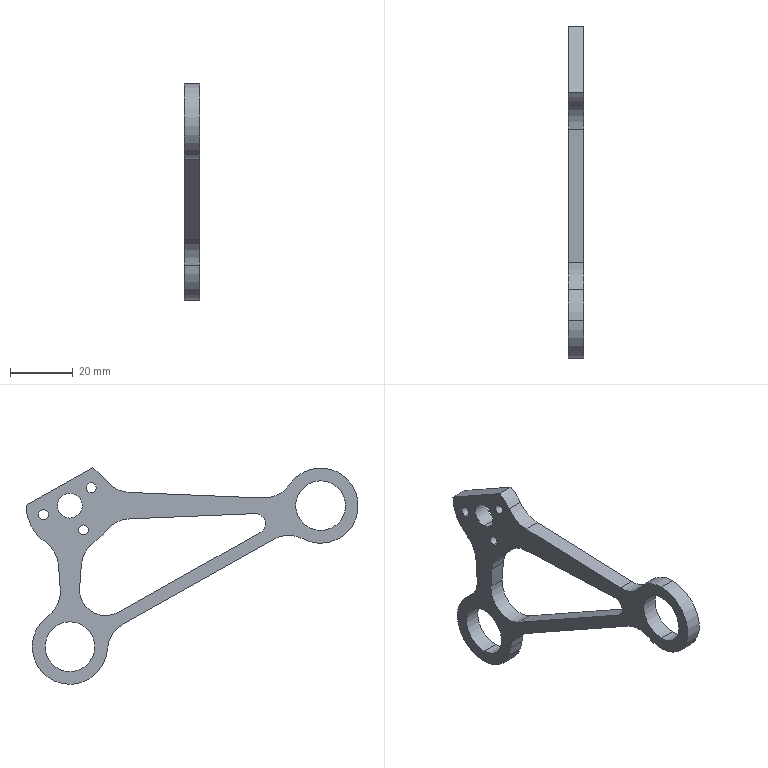Part | SolidWorks | features BaseBody 1 | 1 solid | 40 faces | box 5.08 x 106 x 69.07 mm | volume 9043 mm3 | cylinder 31 | plane 9 | commonest cylinder face diameters 20 x9 3.175 x6 15.875 x4 24 x4 28 x3 6.399 x2
STEP:
#1=CARTESIAN_POINT('',(-2.54,-4.358,-9.336));
#2=VERTEX_POINT('',#1);
#3=CARTESIAN_POINT('',(-2.54,-4.358,-6.161));
#4=VERTEX_POINT('',#3);
#5=CARTESIAN_POINT('',(-2.54,-4.358,-7.748));
#6=DIRECTION('',(-1.,0.,0.));
#7=DIRECTION('',(0.,0.,-1.));
#8=AXIS2_PLACEMENT_3D('',#5,#6,#7);
#9=CIRCLE('',#8,1.588);
#10=EDGE_CURVE('',#2,#4,#9,.T.);
#11=ORIENTED_EDGE('',*,*,#10,.T.);
#12=CARTESIAN_POINT('',(2.54,-4.358,-6.161));
#13=VERTEX_POINT('',#12);
#14=CARTESIAN_POINT('',(-2.54,-4.358,-6.161));
#15=DIRECTION('',(1.,0.,0.));
#16=VECTOR('',#15,1000.);
#17=LINE('',#14,#16);
#18=EDGE_CURVE('',#4,#13,#17,.T.);
#19=ORIENTED_EDGE('',*,*,#18,.T.);
#20=CARTESIAN_POINT('',(2.54,-4.358,-9.336));
#21=VERTEX_POINT('',#20);
#22=CARTESIAN_POINT('',(2.54,-4.358,-7.748));
#23=DIRECTION('',(1.,0.,0.));
#24=DIRECTION('',(0.,0.,-1.));
#25=AXIS2_PLACEMENT_3D('',#22,#23,#24);
#26=CIRCLE('',#25,1.588);
#27=EDGE_CURVE('',#13,#21,#26,.T.);
#28=ORIENTED_EDGE('',*,*,#27,.T.);
#29=CARTESIAN_POINT('',(-2.54,-4.358,-9.336));
#30=DIRECTION('',(1.,0.,0.));
#31=VECTOR('',#30,1000.);
#32=LINE('',#29,#31);
#33=EDGE_CURVE('',#2,#21,#32,.T.);
#34=ORIENTED_EDGE('',*,*,#33,.F.);
#35=EDGE_LOOP('',(#11,#19,#28,#34));
#36=FACE_OUTER_BOUND('',#35,.T.);
#37=CARTESIAN_POINT('',(-2.54,-4.358,-7.748));
#38=DIRECTION('',(1.,0.,0.));
#39=DIRECTION('',(0.,0.,-1.));
#40=AXIS2_PLACEMENT_3D('',#37,#38,#39);
#41=CYLINDRICAL_SURFACE('',#40,1.588);
#42=ADVANCED_FACE('',(#36),#41,.F.);
#43=CARTESIAN_POINT('',(2.54,0.,-52.937));
#44=VERTEX_POINT('',#43);
#45=CARTESIAN_POINT('',(2.54,0.,-37.063));
#46=VERTEX_POINT('',#45);
#47=CARTESIAN_POINT('',(2.54,0.,-45.));
#48=DIRECTION('',(-1.,0.,0.));
#49=DIRECTION('',(0.,0.,1.));
#50=AXIS2_PLACEMENT_3D('',#47,#48,#49);
#51=CIRCLE('',#50,7.937);
#52=EDGE_CURVE('',#44,#46,#51,.T.);
#53=ORIENTED_EDGE('',*,*,#52,.F.);
#54=CARTESIAN_POINT('',(-2.54,0.,-52.937));
#55=VERTEX_POINT('',#54);
#56=CARTESIAN_POINT('',(2.54,0.,-52.937));
#57=DIRECTION('',(-1.,0.,0.));
#58=VECTOR('',#57,1000.);
#59=LINE('',#56,#58);
#60=EDGE_CURVE('',#44,#55,#59,.T.);
#61=ORIENTED_EDGE('',*,*,#60,.T.);
#62=CARTESIAN_POINT('',(-2.54,0.,-37.063));
#63=VERTEX_POINT('',#62);
#64=CARTESIAN_POINT('',(-2.54,0.,-45.));
#65=DIRECTION('',(-1.,0.,0.));
#66=DIRECTION('',(0.,0.,1.));
#67=AXIS2_PLACEMENT_3D('',#64,#65,#66);
#68=CIRCLE('',#67,7.937);
#69=EDGE_CURVE('',#55,#63,#68,.T.);
#70=ORIENTED_EDGE('',*,*,#69,.T.);
#71=CARTESIAN_POINT('',(2.54,0.,-37.063));
#72=DIRECTION('',(-1.,0.,0.));
#73=VECTOR('',#72,1000.);
#74=LINE('',#71,#73);
#75=EDGE_CURVE('',#46,#63,#74,.T.);
#76=ORIENTED_EDGE('',*,*,#75,.F.);
#77=EDGE_LOOP('',(#53,#61,#70,#76));
#78=FACE_OUTER_BOUND('',#77,.T.);
#79=CARTESIAN_POINT('',(2.54,0.,-45.));
#80=DIRECTION('',(-1.,0.,0.));
#81=DIRECTION('',(0.,0.,1.));
#82=AXIS2_PLACEMENT_3D('',#79,#80,#81);
#83=CYLINDRICAL_SURFACE('',#82,7.937);
#84=ADVANCED_FACE('',(#78),#83,.F.);
#85=CARTESIAN_POINT('',(2.54,0.,-3.969));
#86=VERTEX_POINT('',#85);
#87=CARTESIAN_POINT('',(2.54,0.,3.969));
#88=VERTEX_POINT('',#87);
#89=CARTESIAN_POINT('',(2.54,0.,0.));
#90=DIRECTION('',(-1.,0.,0.));
#91=DIRECTION('',(0.,0.,1.));
#92=AXIS2_PLACEMENT_3D('',#89,#90,#91);
#93=CIRCLE('',#92,3.969);
#94=EDGE_CURVE('',#86,#88,#93,.T.);
#95=ORIENTED_EDGE('',*,*,#94,.F.);
#96=CARTESIAN_POINT('',(-2.54,0.,-3.969));
#97=VERTEX_POINT('',#96);
#98=CARTESIAN_POINT('',(2.54,0.,-3.969));
#99=DIRECTION('',(-1.,0.,0.));
#100=VECTOR('',#99,1000.);
#101=LINE('',#98,#100);
#102=EDGE_CURVE('',#86,#97,#101,.T.);
#103=ORIENTED_EDGE('',*,*,#102,.T.);
#104=CARTESIAN_POINT('',(-2.54,0.,3.969));
#105=VERTEX_POINT('',#104);
#106=CARTESIAN_POINT('',(-2.54,0.,0.));
#107=DIRECTION('',(-1.,0.,0.));
#108=DIRECTION('',(0.,0.,1.));
#109=AXIS2_PLACEMENT_3D('',#106,#107,#108);
#110=CIRCLE('',#109,3.969);
#111=EDGE_CURVE('',#97,#105,#110,.T.);
#112=ORIENTED_EDGE('',*,*,#111,.T.);
#113=CARTESIAN_POINT('',(2.54,0.,3.969));
#114=DIRECTION('',(-1.,0.,0.));
#115=VECTOR('',#114,1000.);
#116=LINE('',#113,#115);
#117=EDGE_CURVE('',#88,#105,#116,.T.);
#118=ORIENTED_EDGE('',*,*,#117,.F.);
#119=EDGE_LOOP('',(#95,#103,#112,#118));
#120=FACE_OUTER_BOUND('',#119,.T.);
#121=CARTESIAN_POINT('',(2.54,0.,0.));
#122=DIRECTION('',(-1.,0.,0.));
#123=DIRECTION('',(0.,0.,1.));
#124=AXIS2_PLACEMENT_3D('',#121,#122,#123);
#125=CYLINDRICAL_SURFACE('',#124,3.969);
#126=ADVANCED_FACE('',(#120),#125,.F.);
#127=CARTESIAN_POINT('',(2.54,-59.175,-2.55));
#128=VERTEX_POINT('',#127);
#129=CARTESIAN_POINT('',(2.54,-59.042,-2.552));
#130=VERTEX_POINT('',#129);
#131=CARTESIAN_POINT('',(2.54,-59.175,-5.749));
#132=DIRECTION('',(-1.,0.,0.));
#133=DIRECTION('',(0.,0.,1.));
#134=AXIS2_PLACEMENT_3D('',#131,#132,#133);
#135=CIRCLE('',#134,3.199);
#136=EDGE_CURVE('',#128,#130,#135,.T.);
#137=ORIENTED_EDGE('',*,*,#136,.F.);
#138=CARTESIAN_POINT('',(-2.54,-59.175,-2.55));
#139=VERTEX_POINT('',#138);
#140=CARTESIAN_POINT('',(2.54,-59.175,-2.55));
#141=DIRECTION('',(-1.,0.,0.));
#142=VECTOR('',#141,1000.);
#143=LINE('',#140,#142);
#144=EDGE_CURVE('',#128,#139,#143,.T.);
#145=ORIENTED_EDGE('',*,*,#144,.T.);
#146=CARTESIAN_POINT('',(-2.54,-59.042,-2.552));
#147=VERTEX_POINT('',#146);
#148=CARTESIAN_POINT('',(-2.54,-59.175,-5.749));
#149=DIRECTION('',(-1.,0.,0.));
#150=DIRECTION('',(0.,0.,1.));
#151=AXIS2_PLACEMENT_3D('',#148,#149,#150);
#152=CIRCLE('',#151,3.199);
#153=EDGE_CURVE('',#139,#147,#152,.T.);
#154=ORIENTED_EDGE('',*,*,#153,.T.);
#155=CARTESIAN_POINT('',(0.,-59.042,-2.552));
#156=DIRECTION('',(-1.,0.,0.));
#157=VECTOR('',#156,1000.);
#158=LINE('',#155,#157);
#159=EDGE_CURVE('',#130,#147,#158,.T.);
#160=ORIENTED_EDGE('',*,*,#159,.F.);
#161=EDGE_LOOP('',(#137,#145,#154,#160));
#162=FACE_OUTER_BOUND('',#161,.T.);
#163=CARTESIAN_POINT('',(2.54,-59.175,-5.749));
#164=DIRECTION('',(-1.,0.,0.));
#165=DIRECTION('',(0.,0.,1.));
#166=AXIS2_PLACEMENT_3D('',#163,#164,#165);
#167=CYLINDRICAL_SURFACE('',#166,3.199);
#168=ADVANCED_FACE('',(#162),#167,.F.);
#169=CARTESIAN_POINT('',(2.54,-80.,-7.938));
#170=VERTEX_POINT('',#169);
#171=CARTESIAN_POINT('',(2.54,-80.,7.938));
#172=VERTEX_POINT('',#171);
#173=CARTESIAN_POINT('',(2.54,-80.,0.));
#174=DIRECTION('',(-1.,0.,0.));
#175=DIRECTION('',(0.,0.,1.));
#176=AXIS2_PLACEMENT_3D('',#173,#174,#175);
#177=CIRCLE('',#176,7.938);
#178=EDGE_CURVE('',#170,#172,#177,.T.);
#179=ORIENTED_EDGE('',*,*,#178,.F.);
#180=CARTESIAN_POINT('',(-2.54,-80.,-7.938));
#181=VERTEX_POINT('',#180);
#182=CARTESIAN_POINT('',(2.54,-80.,-7.938));
#183=DIRECTION('',(-1.,0.,0.));
#184=VECTOR('',#183,1000.);
#185=LINE('',#182,#184);
#186=EDGE_CURVE('',#170,#181,#185,.T.);
#187=ORIENTED_EDGE('',*,*,#186,.T.);
#188=CARTESIAN_POINT('',(-2.54,-80.,7.938));
#189=VERTEX_POINT('',#188);
#190=CARTESIAN_POINT('',(-2.54,-80.,0.));
#191=DIRECTION('',(-1.,0.,0.));
#192=DIRECTION('',(0.,0.,1.));
#193=AXIS2_PLACEMENT_3D('',#190,#191,#192);
#194=CIRCLE('',#193,7.938);
#195=EDGE_CURVE('',#181,#189,#194,.T.);
#196=ORIENTED_EDGE('',*,*,#195,.T.);
#197=CARTESIAN_POINT('',(2.54,-80.,7.938));
#198=DIRECTION('',(-1.,0.,0.));
#199=VECTOR('',#198,1000.);
#200=LINE('',#197,#199);
#201=EDGE_CURVE('',#172,#189,#200,.T.);
#202=ORIENTED_EDGE('',*,*,#201,.F.);
#203=EDGE_LOOP('',(#179,#187,#196,#202));
#204=FACE_OUTER_BOUND('',#203,.T.);
#205=CARTESIAN_POINT('',(2.54,-80.,0.));
#206=DIRECTION('',(-1.,0.,0.));
#207=DIRECTION('',(0.,0.,1.));
#208=AXIS2_PLACEMENT_3D('',#205,#206,#207);
#209=CYLINDRICAL_SURFACE('',#208,7.938);
#210=ADVANCED_FACE('',(#204),#209,.F.);
#211=CARTESIAN_POINT('',(-2.54,-6.818,4.117));
#212=VERTEX_POINT('',#211);
#213=CARTESIAN_POINT('',(-2.54,-6.818,7.292));
#214=VERTEX_POINT('',#213);
#215=CARTESIAN_POINT('',(-2.54,-6.818,5.705));
#216=DIRECTION('',(-1.,0.,0.));
#217=DIRECTION('',(0.,0.,-1.));
#218=AXIS2_PLACEMENT_3D('',#215,#216,#217);
#219=CIRCLE('',#218,1.588);
#220=EDGE_CURVE('',#212,#214,#219,.T.);
#221=ORIENTED_EDGE('',*,*,#220,.T.);
#222=CARTESIAN_POINT('',(2.54,-6.818,7.292));
#223=VERTEX_POINT('',#222);
#224=CARTESIAN_POINT('',(-2.54,-6.818,7.292));
#225=DIRECTION('',(1.,0.,0.));
#226=VECTOR('',#225,1000.);
#227=LINE('',#224,#226);
#228=EDGE_CURVE('',#214,#223,#227,.T.);
#229=ORIENTED_EDGE('',*,*,#228,.T.);
#230=CARTESIAN_POINT('',(2.54,-6.818,4.117));
#231=VERTEX_POINT('',#230);
#232=CARTESIAN_POINT('',(2.54,-6.818,5.705));
#233=DIRECTION('',(-1.,0.,0.));
#234=DIRECTION('',(0.,0.,-1.));
#235=AXIS2_PLACEMENT_3D('',#232,#233,#234);
#236=CIRCLE('',#235,1.588);
#237=EDGE_CURVE('',#231,#223,#236,.T.);
#238=ORIENTED_EDGE('',*,*,#237,.F.);
#239=CARTESIAN_POINT('',(-2.54,-6.818,4.117));
#240=DIRECTION('',(1.,0.,0.));
#241=VECTOR('',#240,1000.);
#242=LINE('',#239,#241);
#243=EDGE_CURVE('',#212,#231,#242,.T.);
#244=ORIENTED_EDGE('',*,*,#243,.F.);
#245=EDGE_LOOP('',(#221,#229,#238,#244));
#246=FACE_OUTER_BOUND('',#245,.T.);
#247=CARTESIAN_POINT('',(-2.54,-6.818,5.705));
#248=DIRECTION('',(1.,0.,0.));
#249=DIRECTION('',(0.,0.,-1.));
#250=AXIS2_PLACEMENT_3D('',#247,#248,#249);
#251=CYLINDRICAL_SURFACE('',#250,1.588);
#252=ADVANCED_FACE('',(#246),#251,.F.);
#253=CARTESIAN_POINT('',(-2.54,8.416,-4.452));
#254=VERTEX_POINT('',#253);
#255=CARTESIAN_POINT('',(-2.54,8.416,-1.277));
#256=VERTEX_POINT('',#255);
#257=CARTESIAN_POINT('',(-2.54,8.416,-2.865));
#258=DIRECTION('',(-1.,0.,0.));
#259=DIRECTION('',(0.,0.,-1.));
#260=AXIS2_PLACEMENT_3D('',#257,#258,#259);
#261=CIRCLE('',#260,1.587);
#262=EDGE_CURVE('',#254,#256,#261,.T.);
#263=ORIENTED_EDGE('',*,*,#262,.T.);
#264=CARTESIAN_POINT('',(2.54,8.416,-1.277));
#265=VERTEX_POINT('',#264);
#266=CARTESIAN_POINT('',(-2.54,8.416,-1.277));
#267=DIRECTION('',(1.,0.,0.));
#268=VECTOR('',#267,1000.);
#269=LINE('',#266,#268);
#270=EDGE_CURVE('',#256,#265,#269,.T.);
#271=ORIENTED_EDGE('',*,*,#270,.T.);
#272=CARTESIAN_POINT('',(2.54,8.416,-4.452));
#273=VERTEX_POINT('',#272);
#274=CARTESIAN_POINT('',(2.54,8.416,-2.865));
#275=DIRECTION('',(-1.,0.,0.));
#276=DIRECTION('',(0.,0.,-1.));
#277=AXIS2_PLACEMENT_3D('',#274,#275,#276);
#278=CIRCLE('',#277,1.587);
#279=EDGE_CURVE('',#273,#265,#278,.T.);
#280=ORIENTED_EDGE('',*,*,#279,.F.);
#281=CARTESIAN_POINT('',(-2.54,8.416,-4.452));
#282=DIRECTION('',(1.,0.,0.));
#283=VECTOR('',#282,1000.);
#284=LINE('',#281,#283);
#285=EDGE_CURVE('',#254,#273,#284,.T.);
#286=ORIENTED_EDGE('',*,*,#285,.F.);
#287=EDGE_LOOP('',(#263,#271,#280,#286));
#288=FACE_OUTER_BOUND('',#287,.T.);
#289=CARTESIAN_POINT('',(-2.54,8.416,-2.865));
#290=DIRECTION('',(1.,0.,0.));
#291=DIRECTION('',(0.,0.,-1.));
#292=AXIS2_PLACEMENT_3D('',#289,#290,#291);
#293=CYLINDRICAL_SURFACE('',#292,1.587);
#294=ADVANCED_FACE('',(#288),#293,.F.);
#295=CARTESIAN_POINT('',(2.54,-69.812,-9.499));
#296=VERTEX_POINT('',#295);
#297=CARTESIAN_POINT('',(2.54,-64.909,-10.783));
#298=VERTEX_POINT('',#297);
#299=CARTESIAN_POINT('',(2.54,-69.812,-19.499));
#300=DIRECTION('',(-1.,0.,0.));
#301=DIRECTION('',(0.,0.,1.));
#302=AXIS2_PLACEMENT_3D('',#299,#300,#301);
#303=CIRCLE('',#302,10.);
#304=EDGE_CURVE('',#296,#298,#303,.T.);
#305=ORIENTED_EDGE('',*,*,#304,.F.);
#306=CARTESIAN_POINT('',(-2.54,-69.812,-9.499));
#307=VERTEX_POINT('',#306);
#308=CARTESIAN_POINT('',(2.54,-69.812,-9.499));
#309=DIRECTION('',(-1.,0.,0.));
#310=VECTOR('',#309,1000.);
#311=LINE('',#308,#310);
#312=EDGE_CURVE('',#296,#307,#311,.T.);
#313=ORIENTED_EDGE('',*,*,#312,.T.);
#314=CARTESIAN_POINT('',(-2.54,-64.909,-10.783));
#315=VERTEX_POINT('',#314);
#316=CARTESIAN_POINT('',(-2.54,-69.812,-19.499));
#317=DIRECTION('',(-1.,0.,0.));
#318=DIRECTION('',(0.,0.,1.));
#319=AXIS2_PLACEMENT_3D('',#316,#317,#318);
#320=CIRCLE('',#319,10.);
#321=EDGE_CURVE('',#307,#315,#320,.T.);
#322=ORIENTED_EDGE('',*,*,#321,.T.);
#323=CARTESIAN_POINT('',(0.,-64.909,-10.783));
#324=DIRECTION('',(1.,0.,0.));
#325=VECTOR('',#324,1000.);
#326=LINE('',#323,#325);
#327=EDGE_CURVE('',#315,#298,#326,.T.);
#328=ORIENTED_EDGE('',*,*,#327,.T.);
#329=EDGE_LOOP('',(#305,#313,#322,#328));
#330=FACE_OUTER_BOUND('',#329,.T.);
#331=CARTESIAN_POINT('',(2.54,-69.812,-19.499));
#332=DIRECTION('',(-1.,0.,0.));
#333=DIRECTION('',(0.,0.,1.));
#334=AXIS2_PLACEMENT_3D('',#331,#332,#333);
#335=CYLINDRICAL_SURFACE('',#334,10.);
#336=ADVANCED_FACE('',(#330),#335,.F.);
#337=CARTESIAN_POINT('',(2.54,-80.,-12.));
#338=VERTEX_POINT('',#337);
#339=CARTESIAN_POINT('',(2.54,-74.443,-10.636));
#340=VERTEX_POINT('',#339);
#341=CARTESIAN_POINT('',(2.54,-80.,0.));
#342=DIRECTION('',(1.,0.,0.));
#343=DIRECTION('',(0.,0.,1.));
#344=AXIS2_PLACEMENT_3D('',#341,#342,#343);
#345=CIRCLE('',#344,12.);
#346=EDGE_CURVE('',#338,#340,#345,.T.);
#347=ORIENTED_EDGE('',*,*,#346,.F.);
#348=CARTESIAN_POINT('',(-2.54,-80.,-12.));
#349=VERTEX_POINT('',#348);
#350=CARTESIAN_POINT('',(2.54,-80.,-12.));
#351=DIRECTION('',(-1.,0.,0.));
#352=VECTOR('',#351,1000.);
#353=LINE('',#350,#352);
#354=EDGE_CURVE('',#338,#349,#353,.T.);
#355=ORIENTED_EDGE('',*,*,#354,.T.);
#356=CARTESIAN_POINT('',(-2.54,-74.443,-10.636));
#357=VERTEX_POINT('',#356);
#358=CARTESIAN_POINT('',(-2.54,-80.,0.));
#359=DIRECTION('',(1.,0.,0.));
#360=DIRECTION('',(0.,0.,1.));
#361=AXIS2_PLACEMENT_3D('',#358,#359,#360);
#362=CIRCLE('',#361,12.);
#363=EDGE_CURVE('',#349,#357,#362,.T.);
#364=ORIENTED_EDGE('',*,*,#363,.T.);
#365=CARTESIAN_POINT('',(0.,-74.443,-10.636));
#366=DIRECTION('',(-1.,0.,0.));
#367=VECTOR('',#366,1000.);
#368=LINE('',#365,#367);
#369=EDGE_CURVE('',#340,#357,#368,.T.);
#370=ORIENTED_EDGE('',*,*,#369,.F.);
#371=EDGE_LOOP('',(#347,#355,#364,#370));
#372=FACE_OUTER_BOUND('',#371,.T.);
#373=CARTESIAN_POINT('',(2.54,-80.,0.));
#374=DIRECTION('',(-1.,0.,0.));
#375=DIRECTION('',(0.,0.,1.));
#376=AXIS2_PLACEMENT_3D('',#373,#374,#375);
#377=CYLINDRICAL_SURFACE('',#376,12.);
#378=ADVANCED_FACE('',(#372),#377,.T.);
#379=ORIENTED_EDGE('',*,*,#354,.F.);
#380=CARTESIAN_POINT('',(2.54,-80.,12.));
#381=VERTEX_POINT('',#380);
#382=CARTESIAN_POINT('',(2.54,-80.,0.));
#383=DIRECTION('',(1.,0.,0.));
#384=DIRECTION('',(0.,0.,1.));
#385=AXIS2_PLACEMENT_3D('',#382,#383,#384);
#386=CIRCLE('',#385,12.);
#387=EDGE_CURVE('',#381,#338,#386,.T.);
#388=ORIENTED_EDGE('',*,*,#387,.F.);
#389=CARTESIAN_POINT('',(-2.54,-80.,12.));
#390=VERTEX_POINT('',#389);
#391=CARTESIAN_POINT('',(2.54,-80.,12.));
#392=DIRECTION('',(-1.,0.,0.));
#393=VECTOR('',#392,1000.);
#394=LINE('',#391,#393);
#395=EDGE_CURVE('',#381,#390,#394,.T.);
#396=ORIENTED_EDGE('',*,*,#395,.T.);
#397=CARTESIAN_POINT('',(-2.54,-80.,0.));
#398=DIRECTION('',(1.,0.,0.));
#399=DIRECTION('',(0.,0.,1.));
#400=AXIS2_PLACEMENT_3D('',#397,#398,#399);
#401=CIRCLE('',#400,12.);
#402=EDGE_CURVE('',#390,#349,#401,.T.);
#403=ORIENTED_EDGE('',*,*,#402,.T.);
#404=EDGE_LOOP('',(#379,#388,#396,#403));
#405=FACE_OUTER_BOUND('',#404,.T.);
#406=CARTESIAN_POINT('',(2.54,-80.,0.));
#407=DIRECTION('',(-1.,0.,0.));
#408=DIRECTION('',(0.,0.,1.));
#409=AXIS2_PLACEMENT_3D('',#406,#407,#408);
#410=CYLINDRICAL_SURFACE('',#409,12.);
#411=ADVANCED_FACE('',(#405),#410,.T.);
#412=ORIENTED_EDGE('',*,*,#18,.F.);
#413=CARTESIAN_POINT('',(-2.54,-4.358,-7.748));
#414=DIRECTION('',(-1.,0.,0.));
#415=DIRECTION('',(0.,0.,-1.));
#416=AXIS2_PLACEMENT_3D('',#413,#414,#415);
#417=CIRCLE('',#416,1.588);
#418=EDGE_CURVE('',#4,#2,#417,.T.);
#419=ORIENTED_EDGE('',*,*,#418,.T.);
#420=ORIENTED_EDGE('',*,*,#33,.T.);
#421=CARTESIAN_POINT('',(2.54,-4.358,-7.748));
#422=DIRECTION('',(1.,0.,0.));
#423=DIRECTION('',(0.,0.,-1.));
#424=AXIS2_PLACEMENT_3D('',#421,#422,#423);
#425=CIRCLE('',#424,1.588);
#426=EDGE_CURVE('',#21,#13,#425,.T.);
#427=ORIENTED_EDGE('',*,*,#426,.T.);
#428=EDGE_LOOP('',(#412,#419,#420,#427));
#429=FACE_OUTER_BOUND('',#428,.T.);
#430=CARTESIAN_POINT('',(-2.54,-4.358,-7.748));
#431=DIRECTION('',(1.,0.,0.));
#432=DIRECTION('',(0.,0.,-1.));
#433=AXIS2_PLACEMENT_3D('',#430,#431,#432);
#434=CYLINDRICAL_SURFACE('',#433,1.588);
#435=ADVANCED_FACE('',(#429),#434,.F.);
#436=CARTESIAN_POINT('',(2.54,0.,-45.));
#437=DIRECTION('',(-1.,0.,0.));
#438=DIRECTION('',(0.,0.,1.));
#439=AXIS2_PLACEMENT_3D('',#436,#437,#438);
#440=CIRCLE('',#439,7.937);
#441=EDGE_CURVE('',#46,#44,#440,.T.);
#442=ORIENTED_EDGE('',*,*,#441,.T.);
#443=ORIENTED_EDGE('',*,*,#52,.T.);
#444=EDGE_LOOP('',(#442,#443));
#445=FACE_BOUND('',#444,.T.);
#446=CARTESIAN_POINT('',(2.54,0.,0.));
#447=DIRECTION('',(-1.,0.,0.));
#448=DIRECTION('',(0.,0.,1.));
#449=AXIS2_PLACEMENT_3D('',#446,#447,#448);
#450=CIRCLE('',#449,3.969);
#451=EDGE_CURVE('',#88,#86,#450,.T.);
#452=ORIENTED_EDGE('',*,*,#451,.T.);
#453=ORIENTED_EDGE('',*,*,#94,.T.);
#454=EDGE_LOOP('',(#452,#453));
#455=FACE_BOUND('',#454,.T.);
#456=CARTESIAN_POINT('',(2.54,-11.284,-8.287));
#457=VERTEX_POINT('',#456);
#458=CARTESIAN_POINT('',(2.54,-7.933,-11.536));
#459=VERTEX_POINT('',#458);
#460=CARTESIAN_POINT('',(2.54,0.,0.));
#461=DIRECTION('',(1.,0.,0.));
#462=DIRECTION('',(0.,0.,1.));
#463=AXIS2_PLACEMENT_3D('',#460,#461,#462);
#464=CIRCLE('',#463,14.);
#465=EDGE_CURVE('',#457,#459,#464,.T.);
#466=ORIENTED_EDGE('',*,*,#465,.T.);
#467=CARTESIAN_POINT('',(2.54,-3.625,-19.056));
#468=VERTEX_POINT('',#467);
#469=CARTESIAN_POINT('',(2.54,-13.599,-19.775));
#470=DIRECTION('',(-1.,0.,0.));
#471=DIRECTION('',(0.,0.,1.));
#472=AXIS2_PLACEMENT_3D('',#469,#470,#471);
#473=CIRCLE('',#472,10.);
#474=EDGE_CURVE('',#459,#468,#473,.T.);
#475=ORIENTED_EDGE('',*,*,#474,.T.);
#476=CARTESIAN_POINT('',(2.54,-3.11,-26.192));
#477=VERTEX_POINT('',#476);
#478=CARTESIAN_POINT('',(2.54,-3.625,-19.056));
#479=DIRECTION('',(0.,0.07196,-0.9974));
#480=VECTOR('',#479,1000.);
#481=LINE('',#478,#480);
#482=EDGE_CURVE('',#468,#477,#481,.T.);
#483=ORIENTED_EDGE('',*,*,#482,.T.);
#484=CARTESIAN_POINT('',(2.54,-15.447,-34.017));
#485=VERTEX_POINT('',#484);
#486=CARTESIAN_POINT('',(2.54,-11.381,-26.789));
#487=DIRECTION('',(-1.,0.,0.));
#488=DIRECTION('',(0.,0.,1.));
#489=AXIS2_PLACEMENT_3D('',#486,#487,#488);
#490=CIRCLE('',#489,8.292);
#491=EDGE_CURVE('',#477,#485,#490,.T.);
#492=ORIENTED_EDGE('',*,*,#491,.T.);
#493=CARTESIAN_POINT('',(2.54,-60.743,-8.537));
#494=VERTEX_POINT('',#493);
#495=CARTESIAN_POINT('',(2.54,-15.447,-34.017));
#496=DIRECTION('',(0.,-0.8716,0.4903));
#497=VECTOR('',#496,1000.);
#498=LINE('',#495,#497);
#499=EDGE_CURVE('',#485,#494,#498,.T.);
#500=ORIENTED_EDGE('',*,*,#499,.T.);
#501=CARTESIAN_POINT('',(2.54,-59.175,-5.749));
#502=DIRECTION('',(-1.,0.,0.));
#503=DIRECTION('',(0.,0.,1.));
#504=AXIS2_PLACEMENT_3D('',#501,#502,#503);
#505=CIRCLE('',#504,3.199);
#506=EDGE_CURVE('',#494,#128,#505,.T.);
#507=ORIENTED_EDGE('',*,*,#506,.T.);
#508=ORIENTED_EDGE('',*,*,#136,.T.);
#509=CARTESIAN_POINT('',(2.54,-18.929,-4.215));
#510=VERTEX_POINT('',#509);
#511=CARTESIAN_POINT('',(2.54,-59.042,-2.552));
#512=DIRECTION('',(0.,0.9991,-0.04142));
#513=VECTOR('',#512,1000.);
#514=LINE('',#511,#513);
#515=EDGE_CURVE('',#130,#510,#514,.T.);
#516=ORIENTED_EDGE('',*,*,#515,.T.);
#517=CARTESIAN_POINT('',(2.54,-19.343,-14.207));
#518=DIRECTION('',(-1.,0.,0.));
#519=DIRECTION('',(0.,0.,1.));
#520=AXIS2_PLACEMENT_3D('',#517,#518,#519);
#521=CIRCLE('',#520,10.);
#522=EDGE_CURVE('',#510,#457,#521,.T.);
#523=ORIENTED_EDGE('',*,*,#522,.T.);
#524=EDGE_LOOP('',(#466,#475,#483,#492,#500,#507,#508,#516,#523));
#525=FACE_BOUND('',#524,.T.);
#526=CARTESIAN_POINT('',(2.54,-80.,0.));
#527=DIRECTION('',(-1.,0.,0.));
#528=DIRECTION('',(0.,0.,1.));
#529=AXIS2_PLACEMENT_3D('',#526,#527,#528);
#530=CIRCLE('',#529,7.938);
#531=EDGE_CURVE('',#172,#170,#530,.T.);
#532=ORIENTED_EDGE('',*,*,#531,.T.);
#533=ORIENTED_EDGE('',*,*,#178,.T.);
#534=EDGE_LOOP('',(#532,#533));
#535=FACE_BOUND('',#534,.T.);
#536=ORIENTED_EDGE('',*,*,#237,.T.);
#537=CARTESIAN_POINT('',(2.54,-6.818,5.705));
#538=DIRECTION('',(-1.,0.,0.));
#539=DIRECTION('',(0.,0.,-1.));
#540=AXIS2_PLACEMENT_3D('',#537,#538,#539);
#541=CIRCLE('',#540,1.588);
#542=EDGE_CURVE('',#223,#231,#541,.T.);
#543=ORIENTED_EDGE('',*,*,#542,.T.);
#544=EDGE_LOOP('',(#536,#543));
#545=FACE_BOUND('',#544,.T.);
#546=ORIENTED_EDGE('',*,*,#279,.T.);
#547=CARTESIAN_POINT('',(2.54,8.416,-2.865));
#548=DIRECTION('',(-1.,0.,0.));
#549=DIRECTION('',(0.,0.,-1.));
#550=AXIS2_PLACEMENT_3D('',#547,#548,#549);
#551=CIRCLE('',#550,1.587);
#552=EDGE_CURVE('',#265,#273,#551,.T.);
#553=ORIENTED_EDGE('',*,*,#552,.T.);
#554=EDGE_LOOP('',(#546,#553));
#555=FACE_BOUND('',#554,.T.);
#556=ORIENTED_EDGE('',*,*,#426,.F.);
#557=ORIENTED_EDGE('',*,*,#27,.F.);
#558=EDGE_LOOP('',(#556,#557));
#559=FACE_BOUND('',#558,.T.);
#560=CARTESIAN_POINT('',(2.54,3.625,-19.056));
#561=VERTEX_POINT('',#560);
#562=CARTESIAN_POINT('',(2.54,7.933,-11.536));
#563=VERTEX_POINT('',#562);
#564=CARTESIAN_POINT('',(2.54,13.599,-19.775));
#565=DIRECTION('',(-1.,0.,0.));
#566=DIRECTION('',(0.,0.,1.));
#567=AXIS2_PLACEMENT_3D('',#564,#565,#566);
#568=CIRCLE('',#567,10.);
#569=EDGE_CURVE('',#561,#563,#568,.T.);
#570=ORIENTED_EDGE('',*,*,#569,.T.);
#571=CARTESIAN_POINT('',(2.54,13.998,0.2051));
#572=VERTEX_POINT('',#571);
#573=CARTESIAN_POINT('',(2.54,0.,0.));
#574=DIRECTION('',(1.,0.,0.));
#575=DIRECTION('',(0.,0.,1.));
#576=AXIS2_PLACEMENT_3D('',#573,#574,#575);
#577=CIRCLE('',#576,14.);
#578=EDGE_CURVE('',#563,#572,#577,.T.);
#579=ORIENTED_EDGE('',*,*,#578,.T.);
#580=CARTESIAN_POINT('',(2.54,-7.094,12.07));
#581=VERTEX_POINT('',#580);
#582=CARTESIAN_POINT('',(2.54,13.998,0.2051));
#583=DIRECTION('',(0.,-0.8716,0.4903));
#584=VECTOR('',#583,1000.);
#585=LINE('',#582,#584);
#586=EDGE_CURVE('',#572,#581,#585,.T.);
#587=ORIENTED_EDGE('',*,*,#586,.T.);
#588=CARTESIAN_POINT('',(2.54,-11.284,8.287));
#589=VERTEX_POINT('',#588);
#590=CARTESIAN_POINT('',(2.54,0.,0.));
#591=DIRECTION('',(1.,0.,0.));
#592=DIRECTION('',(0.,0.,1.));
#593=AXIS2_PLACEMENT_3D('',#590,#591,#592);
#594=CIRCLE('',#593,14.);
#595=EDGE_CURVE('',#581,#589,#594,.T.);
#596=ORIENTED_EDGE('',*,*,#595,.T.);
#597=CARTESIAN_POINT('',(2.54,-18.929,4.215));
#598=VERTEX_POINT('',#597);
#599=CARTESIAN_POINT('',(2.54,-19.343,14.207));
#600=DIRECTION('',(-1.,0.,0.));
#601=DIRECTION('',(0.,0.,1.));
#602=AXIS2_PLACEMENT_3D('',#599,#600,#601);
#603=CIRCLE('',#602,10.);
#604=EDGE_CURVE('',#589,#598,#603,.T.);
#605=ORIENTED_EDGE('',*,*,#604,.T.);
#606=CARTESIAN_POINT('',(2.54,-61.444,2.453));
#607=VERTEX_POINT('',#606);
#608=CARTESIAN_POINT('',(2.54,-18.929,4.215));
#609=DIRECTION('',(0.,-0.9991,-0.04142));
#610=VECTOR('',#609,1000.);
#611=LINE('',#608,#610);
#612=EDGE_CURVE('',#598,#607,#611,.T.);
#613=ORIENTED_EDGE('',*,*,#612,.T.);
#614=CARTESIAN_POINT('',(2.54,-70.104,6.788));
#615=VERTEX_POINT('',#614);
#616=CARTESIAN_POINT('',(2.54,-61.858,12.444));
#617=DIRECTION('',(-1.,0.,0.));
#618=DIRECTION('',(0.,0.,1.));
#619=AXIS2_PLACEMENT_3D('',#616,#617,#618);
#620=CIRCLE('',#619,10.);
#621=EDGE_CURVE('',#607,#615,#620,.T.);
#622=ORIENTED_EDGE('',*,*,#621,.T.);
#623=CARTESIAN_POINT('',(2.54,-80.,0.));
#624=DIRECTION('',(1.,0.,0.));
#625=DIRECTION('',(0.,0.,1.));
#626=AXIS2_PLACEMENT_3D('',#623,#624,#625);
#627=CIRCLE('',#626,12.);
#628=EDGE_CURVE('',#615,#381,#627,.T.);
#629=ORIENTED_EDGE('',*,*,#628,.T.);
#630=ORIENTED_EDGE('',*,*,#387,.T.);
#631=ORIENTED_EDGE('',*,*,#346,.T.);
#632=CARTESIAN_POINT('',(2.54,-69.812,-19.499));
#633=DIRECTION('',(-1.,0.,0.));
#634=DIRECTION('',(0.,0.,1.));
#635=AXIS2_PLACEMENT_3D('',#632,#633,#634);
#636=CIRCLE('',#635,10.);
#637=EDGE_CURVE('',#340,#296,#636,.T.);
#638=ORIENTED_EDGE('',*,*,#637,.T.);
#639=ORIENTED_EDGE('',*,*,#304,.T.);
#640=CARTESIAN_POINT('',(2.54,-17.052,-37.703));
#641=VERTEX_POINT('',#640);
#642=CARTESIAN_POINT('',(2.54,-64.909,-10.783));
#643=DIRECTION('',(0.,0.8716,-0.4903));
#644=VECTOR('',#643,1000.);
#645=LINE('',#642,#644);
#646=EDGE_CURVE('',#298,#641,#645,.T.);
#647=ORIENTED_EDGE('',*,*,#646,.T.);
#648=CARTESIAN_POINT('',(2.54,-11.975,-45.774));
#649=VERTEX_POINT('',#648);
#650=CARTESIAN_POINT('',(2.54,-21.954,-46.419));
#651=DIRECTION('',(-1.,0.,0.));
#652=DIRECTION('',(0.,0.,1.));
#653=AXIS2_PLACEMENT_3D('',#650,#651,#652);
#654=CIRCLE('',#653,10.);
#655=EDGE_CURVE('',#641,#649,#654,.T.);
#656=ORIENTED_EDGE('',*,*,#655,.T.);
#657=CARTESIAN_POINT('',(2.54,7.122,-35.342));
#658=VERTEX_POINT('',#657);
#659=CARTESIAN_POINT('',(2.54,0.,-45.));
#660=DIRECTION('',(1.,0.,0.));
#661=DIRECTION('',(0.,0.,1.));
#662=AXIS2_PLACEMENT_3D('',#659,#660,#661);
#663=CIRCLE('',#662,12.);
#664=EDGE_CURVE('',#649,#658,#663,.T.);
#665=ORIENTED_EDGE('',*,*,#664,.T.);
#666=CARTESIAN_POINT('',(2.54,3.083,-26.574));
#667=VERTEX_POINT('',#666);
#668=CARTESIAN_POINT('',(2.54,13.057,-27.293));
#669=DIRECTION('',(-1.,0.,0.));
#670=DIRECTION('',(0.,0.,1.));
#671=AXIS2_PLACEMENT_3D('',#668,#669,#670);
#672=CIRCLE('',#671,10.);
#673=EDGE_CURVE('',#658,#667,#672,.T.);
#674=ORIENTED_EDGE('',*,*,#673,.T.);
#675=CARTESIAN_POINT('',(2.54,3.083,-26.574));
#676=DIRECTION('',(0.,0.07196,0.9974));
#677=VECTOR('',#676,1000.);
#678=LINE('',#675,#677);
#679=EDGE_CURVE('',#667,#561,#678,.T.);
#680=ORIENTED_EDGE('',*,*,#679,.T.);
#681=EDGE_LOOP('',(#570,#579,#587,#596,#605,#613,#622,#629,#630,#631,#638,#639,#647,#656,#665,#674,#680));
#682=FACE_OUTER_BOUND('',#681,.T.);
#683=CARTESIAN_POINT('',(2.54,-92.636,12.484));
#684=DIRECTION('',(1.,0.,0.));
#685=DIRECTION('',(0.,0.,-1.));
#686=AXIS2_PLACEMENT_3D('',#683,#684,#685);
#687=PLANE('',#686);
#688=ADVANCED_FACE('',(#445,#455,#525,#535,#545,#555,#559,#682),#687,.T.);
#689=CARTESIAN_POINT('',(-2.54,0.,-45.));
#690=DIRECTION('',(-1.,0.,0.));
#691=DIRECTION('',(0.,0.,1.));
#692=AXIS2_PLACEMENT_3D('',#689,#690,#691);
#693=CIRCLE('',#692,7.937);
#694=EDGE_CURVE('',#63,#55,#693,.T.);
#695=ORIENTED_EDGE('',*,*,#694,.F.);
#696=ORIENTED_EDGE('',*,*,#69,.F.);
#697=EDGE_LOOP('',(#695,#696));
#698=FACE_BOUND('',#697,.T.);
#699=CARTESIAN_POINT('',(-2.54,0.,0.));
#700=DIRECTION('',(-1.,0.,0.));
#701=DIRECTION('',(0.,0.,1.));
#702=AXIS2_PLACEMENT_3D('',#699,#700,#701);
#703=CIRCLE('',#702,3.969);
#704=EDGE_CURVE('',#105,#97,#703,.T.);
#705=ORIENTED_EDGE('',*,*,#704,.F.);
#706=ORIENTED_EDGE('',*,*,#111,.F.);
#707=EDGE_LOOP('',(#705,#706));
#708=FACE_BOUND('',#707,.T.);
#709=CARTESIAN_POINT('',(-2.54,-3.625,-19.056));
#710=VERTEX_POINT('',#709);
#711=CARTESIAN_POINT('',(-2.54,-3.11,-26.192));
#712=VERTEX_POINT('',#711);
#713=CARTESIAN_POINT('',(-2.54,-3.625,-19.056));
#714=DIRECTION('',(0.,0.07196,-0.9974));
#715=VECTOR('',#714,1000.);
#716=LINE('',#713,#715);
#717=EDGE_CURVE('',#710,#712,#716,.T.);
#718=ORIENTED_EDGE('',*,*,#717,.F.);
#719=CARTESIAN_POINT('',(-2.54,-7.933,-11.536));
#720=VERTEX_POINT('',#719);
#721=CARTESIAN_POINT('',(-2.54,-13.599,-19.775));
#722=DIRECTION('',(-1.,0.,0.));
#723=DIRECTION('',(0.,0.,1.));
#724=AXIS2_PLACEMENT_3D('',#721,#722,#723);
#725=CIRCLE('',#724,10.);
#726=EDGE_CURVE('',#720,#710,#725,.T.);
#727=ORIENTED_EDGE('',*,*,#726,.F.);
#728=CARTESIAN_POINT('',(-2.54,-11.284,-8.287));
#729=VERTEX_POINT('',#728);
#730=CARTESIAN_POINT('',(-2.54,0.,0.));
#731=DIRECTION('',(1.,0.,0.));
#732=DIRECTION('',(0.,0.,1.));
#733=AXIS2_PLACEMENT_3D('',#730,#731,#732);
#734=CIRCLE('',#733,14.);
#735=EDGE_CURVE('',#729,#720,#734,.T.);
#736=ORIENTED_EDGE('',*,*,#735,.F.);
#737=CARTESIAN_POINT('',(-2.54,-18.929,-4.215));
#738=VERTEX_POINT('',#737);
#739=CARTESIAN_POINT('',(-2.54,-19.343,-14.207));
#740=DIRECTION('',(-1.,0.,0.));
#741=DIRECTION('',(0.,0.,1.));
#742=AXIS2_PLACEMENT_3D('',#739,#740,#741);
#743=CIRCLE('',#742,10.);
#744=EDGE_CURVE('',#738,#729,#743,.T.);
#745=ORIENTED_EDGE('',*,*,#744,.F.);
#746=CARTESIAN_POINT('',(-2.54,-59.042,-2.552));
#747=DIRECTION('',(0.,0.9991,-0.04142));
#748=VECTOR('',#747,1000.);
#749=LINE('',#746,#748);
#750=EDGE_CURVE('',#147,#738,#749,.T.);
#751=ORIENTED_EDGE('',*,*,#750,.F.);
#752=ORIENTED_EDGE('',*,*,#153,.F.);
#753=CARTESIAN_POINT('',(-2.54,-60.743,-8.537));
#754=VERTEX_POINT('',#753);
#755=CARTESIAN_POINT('',(-2.54,-59.175,-5.749));
#756=DIRECTION('',(-1.,0.,0.));
#757=DIRECTION('',(0.,0.,1.));
#758=AXIS2_PLACEMENT_3D('',#755,#756,#757);
#759=CIRCLE('',#758,3.199);
#760=EDGE_CURVE('',#754,#139,#759,.T.);
#761=ORIENTED_EDGE('',*,*,#760,.F.);
#762=CARTESIAN_POINT('',(-2.54,-15.447,-34.017));
#763=VERTEX_POINT('',#762);
#764=CARTESIAN_POINT('',(-2.54,-15.447,-34.017));
#765=DIRECTION('',(0.,-0.8716,0.4903));
#766=VECTOR('',#765,1000.);
#767=LINE('',#764,#766);
#768=EDGE_CURVE('',#763,#754,#767,.T.);
#769=ORIENTED_EDGE('',*,*,#768,.F.);
#770=CARTESIAN_POINT('',(-2.54,-11.381,-26.789));
#771=DIRECTION('',(-1.,0.,0.));
#772=DIRECTION('',(0.,0.,1.));
#773=AXIS2_PLACEMENT_3D('',#770,#771,#772);
#774=CIRCLE('',#773,8.292);
#775=EDGE_CURVE('',#712,#763,#774,.T.);
#776=ORIENTED_EDGE('',*,*,#775,.F.);
#777=EDGE_LOOP('',(#718,#727,#736,#745,#751,#752,#761,#769,#776));
#778=FACE_BOUND('',#777,.T.);
#779=CARTESIAN_POINT('',(-2.54,-80.,0.));
#780=DIRECTION('',(-1.,0.,0.));
#781=DIRECTION('',(0.,0.,1.));
#782=AXIS2_PLACEMENT_3D('',#779,#780,#781);
#783=CIRCLE('',#782,7.938);
#784=EDGE_CURVE('',#189,#181,#783,.T.);
#785=ORIENTED_EDGE('',*,*,#784,.F.);
#786=ORIENTED_EDGE('',*,*,#195,.F.);
#787=EDGE_LOOP('',(#785,#786));
#788=FACE_BOUND('',#787,.T.);
#789=ORIENTED_EDGE('',*,*,#220,.F.);
#790=CARTESIAN_POINT('',(-2.54,-6.818,5.705));
#791=DIRECTION('',(-1.,0.,0.));
#792=DIRECTION('',(0.,0.,-1.));
#793=AXIS2_PLACEMENT_3D('',#790,#791,#792);
#794=CIRCLE('',#793,1.588);
#795=EDGE_CURVE('',#214,#212,#794,.T.);
#796=ORIENTED_EDGE('',*,*,#795,.F.);
#797=EDGE_LOOP('',(#789,#796));
#798=FACE_BOUND('',#797,.T.);
#799=ORIENTED_EDGE('',*,*,#262,.F.);
#800=CARTESIAN_POINT('',(-2.54,8.416,-2.865));
#801=DIRECTION('',(-1.,0.,0.));
#802=DIRECTION('',(0.,0.,-1.));
#803=AXIS2_PLACEMENT_3D('',#800,#801,#802);
#804=CIRCLE('',#803,1.587);
#805=EDGE_CURVE('',#256,#254,#804,.T.);
#806=ORIENTED_EDGE('',*,*,#805,.F.);
#807=EDGE_LOOP('',(#799,#806));
#808=FACE_BOUND('',#807,.T.);
#809=ORIENTED_EDGE('',*,*,#10,.F.);
#810=ORIENTED_EDGE('',*,*,#418,.F.);
#811=EDGE_LOOP('',(#809,#810));
#812=FACE_BOUND('',#811,.T.);
#813=CARTESIAN_POINT('',(-2.54,13.998,0.2051));
#814=VERTEX_POINT('',#813);
#815=CARTESIAN_POINT('',(-2.54,-7.094,12.07));
#816=VERTEX_POINT('',#815);
#817=CARTESIAN_POINT('',(-2.54,-7.094,12.07));
#818=DIRECTION('',(0.,-0.8716,0.4903));
#819=VECTOR('',#818,1000.);
#820=LINE('',#817,#819);
#821=EDGE_CURVE('',#814,#816,#820,.T.);
#822=ORIENTED_EDGE('',*,*,#821,.F.);
#823=CARTESIAN_POINT('',(-2.54,7.933,-11.536));
#824=VERTEX_POINT('',#823);
#825=CARTESIAN_POINT('',(-2.54,0.,0.));
#826=DIRECTION('',(1.,0.,0.));
#827=DIRECTION('',(0.,0.,1.));
#828=AXIS2_PLACEMENT_3D('',#825,#826,#827);
#829=CIRCLE('',#828,14.);
#830=EDGE_CURVE('',#824,#814,#829,.T.);
#831=ORIENTED_EDGE('',*,*,#830,.F.);
#832=CARTESIAN_POINT('',(-2.54,3.625,-19.056));
#833=VERTEX_POINT('',#832);
#834=CARTESIAN_POINT('',(-2.54,13.599,-19.775));
#835=DIRECTION('',(-1.,0.,0.));
#836=DIRECTION('',(0.,0.,1.));
#837=AXIS2_PLACEMENT_3D('',#834,#835,#836);
#838=CIRCLE('',#837,10.);
#839=EDGE_CURVE('',#833,#824,#838,.T.);
#840=ORIENTED_EDGE('',*,*,#839,.F.);
#841=CARTESIAN_POINT('',(-2.54,3.083,-26.574));
#842=VERTEX_POINT('',#841);
#843=CARTESIAN_POINT('',(-2.54,3.625,-19.056));
#844=DIRECTION('',(0.,0.07196,0.9974));
#845=VECTOR('',#844,1000.);
#846=LINE('',#843,#845);
#847=EDGE_CURVE('',#842,#833,#846,.T.);
#848=ORIENTED_EDGE('',*,*,#847,.F.);
#849=CARTESIAN_POINT('',(-2.54,7.122,-35.342));
#850=VERTEX_POINT('',#849);
#851=CARTESIAN_POINT('',(-2.54,13.057,-27.293));
#852=DIRECTION('',(-1.,0.,0.));
#853=DIRECTION('',(0.,0.,1.));
#854=AXIS2_PLACEMENT_3D('',#851,#852,#853);
#855=CIRCLE('',#854,10.);
#856=EDGE_CURVE('',#850,#842,#855,.T.);
#857=ORIENTED_EDGE('',*,*,#856,.F.);
#858=CARTESIAN_POINT('',(-2.54,-11.975,-45.774));
#859=VERTEX_POINT('',#858);
#860=CARTESIAN_POINT('',(-2.54,0.,-45.));
#861=DIRECTION('',(1.,0.,0.));
#862=DIRECTION('',(0.,0.,1.));
#863=AXIS2_PLACEMENT_3D('',#860,#861,#862);
#864=CIRCLE('',#863,12.);
#865=EDGE_CURVE('',#859,#850,#864,.T.);
#866=ORIENTED_EDGE('',*,*,#865,.F.);
#867=CARTESIAN_POINT('',(-2.54,-17.052,-37.703));
#868=VERTEX_POINT('',#867);
#869=CARTESIAN_POINT('',(-2.54,-21.954,-46.419));
#870=DIRECTION('',(-1.,0.,0.));
#871=DIRECTION('',(0.,0.,1.));
#872=AXIS2_PLACEMENT_3D('',#869,#870,#871);
#873=CIRCLE('',#872,10.);
#874=EDGE_CURVE('',#868,#859,#873,.T.);
#875=ORIENTED_EDGE('',*,*,#874,.F.);
#876=CARTESIAN_POINT('',(-2.54,-17.052,-37.703));
#877=DIRECTION('',(0.,0.8716,-0.4903));
#878=VECTOR('',#877,1000.);
#879=LINE('',#876,#878);
#880=EDGE_CURVE('',#315,#868,#879,.T.);
#881=ORIENTED_EDGE('',*,*,#880,.F.);
#882=ORIENTED_EDGE('',*,*,#321,.F.);
#883=CARTESIAN_POINT('',(-2.54,-69.812,-19.499));
#884=DIRECTION('',(-1.,0.,0.));
#885=DIRECTION('',(0.,0.,1.));
#886=AXIS2_PLACEMENT_3D('',#883,#884,#885);
#887=CIRCLE('',#886,10.);
#888=EDGE_CURVE('',#357,#307,#887,.T.);
#889=ORIENTED_EDGE('',*,*,#888,.F.);
#890=ORIENTED_EDGE('',*,*,#363,.F.);
#891=ORIENTED_EDGE('',*,*,#402,.F.);
#892=CARTESIAN_POINT('',(-2.54,-70.104,6.788));
#893=VERTEX_POINT('',#892);
#894=CARTESIAN_POINT('',(-2.54,-80.,0.));
#895=DIRECTION('',(1.,0.,0.));
#896=DIRECTION('',(0.,0.,1.));
#897=AXIS2_PLACEMENT_3D('',#894,#895,#896);
#898=CIRCLE('',#897,12.);
#899=EDGE_CURVE('',#893,#390,#898,.T.);
#900=ORIENTED_EDGE('',*,*,#899,.F.);
#901=CARTESIAN_POINT('',(-2.54,-61.444,2.453));
#902=VERTEX_POINT('',#901);
#903=CARTESIAN_POINT('',(-2.54,-61.858,12.444));
#904=DIRECTION('',(-1.,0.,0.));
#905=DIRECTION('',(0.,0.,1.));
#906=AXIS2_PLACEMENT_3D('',#903,#904,#905);
#907=CIRCLE('',#906,10.);
#908=EDGE_CURVE('',#902,#893,#907,.T.);
#909=ORIENTED_EDGE('',*,*,#908,.F.);
#910=CARTESIAN_POINT('',(-2.54,-18.929,4.215));
#911=VERTEX_POINT('',#910);
#912=CARTESIAN_POINT('',(-2.54,-61.444,2.453));
#913=DIRECTION('',(0.,-0.9991,-0.04142));
#914=VECTOR('',#913,1000.);
#915=LINE('',#912,#914);
#916=EDGE_CURVE('',#911,#902,#915,.T.);
#917=ORIENTED_EDGE('',*,*,#916,.F.);
#918=CARTESIAN_POINT('',(-2.54,-11.284,8.287));
#919=VERTEX_POINT('',#918);
#920=CARTESIAN_POINT('',(-2.54,-19.343,14.207));
#921=DIRECTION('',(-1.,0.,0.));
#922=DIRECTION('',(0.,0.,1.));
#923=AXIS2_PLACEMENT_3D('',#920,#921,#922);
#924=CIRCLE('',#923,10.);
#925=EDGE_CURVE('',#919,#911,#924,.T.);
#926=ORIENTED_EDGE('',*,*,#925,.F.);
#927=CARTESIAN_POINT('',(-2.54,0.,0.));
#928=DIRECTION('',(1.,0.,0.));
#929=DIRECTION('',(0.,0.,1.));
#930=AXIS2_PLACEMENT_3D('',#927,#928,#929);
#931=CIRCLE('',#930,14.);
#932=EDGE_CURVE('',#816,#919,#931,.T.);
#933=ORIENTED_EDGE('',*,*,#932,.F.);
#934=EDGE_LOOP('',(#822,#831,#840,#848,#857,#866,#875,#881,#882,#889,#890,#891,#900,#909,#917,#926,#933));
#935=FACE_OUTER_BOUND('',#934,.T.);
#936=CARTESIAN_POINT('',(-2.54,-92.636,12.484));
#937=DIRECTION('',(1.,0.,0.));
#938=DIRECTION('',(0.,0.,-1.));
#939=AXIS2_PLACEMENT_3D('',#936,#937,#938);
#940=PLANE('',#939);
#941=ADVANCED_FACE('',(#698,#708,#778,#788,#798,#808,#812,#935),#940,.F.);
#942=ORIENTED_EDGE('',*,*,#60,.F.);
#943=ORIENTED_EDGE('',*,*,#441,.F.);
#944=ORIENTED_EDGE('',*,*,#75,.T.);
#945=ORIENTED_EDGE('',*,*,#694,.T.);
#946=EDGE_LOOP('',(#942,#943,#944,#945));
#947=FACE_OUTER_BOUND('',#946,.T.);
#948=CARTESIAN_POINT('',(2.54,0.,-45.));
#949=DIRECTION('',(-1.,0.,0.));
#950=DIRECTION('',(0.,0.,1.));
#951=AXIS2_PLACEMENT_3D('',#948,#949,#950);
#952=CYLINDRICAL_SURFACE('',#951,7.937);
#953=ADVANCED_FACE('',(#947),#952,.F.);
#954=ORIENTED_EDGE('',*,*,#102,.F.);
#955=ORIENTED_EDGE('',*,*,#451,.F.);
#956=ORIENTED_EDGE('',*,*,#117,.T.);
#957=ORIENTED_EDGE('',*,*,#704,.T.);
#958=EDGE_LOOP('',(#954,#955,#956,#957));
#959=FACE_OUTER_BOUND('',#958,.T.);
#960=CARTESIAN_POINT('',(2.54,0.,0.));
#961=DIRECTION('',(-1.,0.,0.));
#962=DIRECTION('',(0.,0.,1.));
#963=AXIS2_PLACEMENT_3D('',#960,#961,#962);
#964=CYLINDRICAL_SURFACE('',#963,3.969);
#965=ADVANCED_FACE('',(#959),#964,.F.);
#966=ORIENTED_EDGE('',*,*,#474,.F.);
#967=CARTESIAN_POINT('',(0.,-7.933,-11.536));
#968=DIRECTION('',(-1.,0.,0.));
#969=VECTOR('',#968,1000.);
#970=LINE('',#967,#969);
#971=EDGE_CURVE('',#459,#720,#970,.T.);
#972=ORIENTED_EDGE('',*,*,#971,.T.);
#973=ORIENTED_EDGE('',*,*,#726,.T.);
#974=CARTESIAN_POINT('',(0.,-3.625,-19.056));
#975=DIRECTION('',(1.,0.,0.));
#976=VECTOR('',#975,1000.);
#977=LINE('',#974,#976);
#978=EDGE_CURVE('',#710,#468,#977,.T.);
#979=ORIENTED_EDGE('',*,*,#978,.T.);
#980=EDGE_LOOP('',(#966,#972,#973,#979));
#981=FACE_OUTER_BOUND('',#980,.T.);
#982=CARTESIAN_POINT('',(2.54,-13.599,-19.775));
#983=DIRECTION('',(-1.,0.,0.));
#984=DIRECTION('',(0.,0.,1.));
#985=AXIS2_PLACEMENT_3D('',#982,#983,#984);
#986=CYLINDRICAL_SURFACE('',#985,10.);
#987=ADVANCED_FACE('',(#981),#986,.F.);
#988=ORIENTED_EDGE('',*,*,#971,.F.);
#989=ORIENTED_EDGE('',*,*,#465,.F.);
#990=CARTESIAN_POINT('',(0.,-11.284,-8.287));
#991=DIRECTION('',(1.,0.,0.));
#992=VECTOR('',#991,1000.);
#993=LINE('',#990,#992);
#994=EDGE_CURVE('',#729,#457,#993,.T.);
#995=ORIENTED_EDGE('',*,*,#994,.F.);
#996=ORIENTED_EDGE('',*,*,#735,.T.);
#997=EDGE_LOOP('',(#988,#989,#995,#996));
#998=FACE_OUTER_BOUND('',#997,.T.);
#999=CARTESIAN_POINT('',(2.54,0.,0.));
#1000=DIRECTION('',(-1.,0.,0.));
#1001=DIRECTION('',(0.,0.,1.));
#1002=AXIS2_PLACEMENT_3D('',#999,#1000,#1001);
#1003=CYLINDRICAL_SURFACE('',#1002,14.);
#1004=ADVANCED_FACE('',(#998),#1003,.T.);
#1005=ORIENTED_EDGE('',*,*,#522,.F.);
#1006=CARTESIAN_POINT('',(0.,-18.929,-4.215));
#1007=DIRECTION('',(-1.,0.,0.));
#1008=VECTOR('',#1007,1000.);
#1009=LINE('',#1006,#1008);
#1010=EDGE_CURVE('',#510,#738,#1009,.T.);
#1011=ORIENTED_EDGE('',*,*,#1010,.T.);
#1012=ORIENTED_EDGE('',*,*,#744,.T.);
#1013=ORIENTED_EDGE('',*,*,#994,.T.);
#1014=EDGE_LOOP('',(#1005,#1011,#1012,#1013));
#1015=FACE_OUTER_BOUND('',#1014,.T.);
#1016=CARTESIAN_POINT('',(2.54,-19.343,-14.207));
#1017=DIRECTION('',(-1.,0.,0.));
#1018=DIRECTION('',(0.,0.,1.));
#1019=AXIS2_PLACEMENT_3D('',#1016,#1017,#1018);
#1020=CYLINDRICAL_SURFACE('',#1019,10.);
#1021=ADVANCED_FACE('',(#1015),#1020,.F.);
#1022=ORIENTED_EDGE('',*,*,#515,.F.);
#1023=ORIENTED_EDGE('',*,*,#159,.T.);
#1024=ORIENTED_EDGE('',*,*,#750,.T.);
#1025=ORIENTED_EDGE('',*,*,#1010,.F.);
#1026=EDGE_LOOP('',(#1022,#1023,#1024,#1025));
#1027=FACE_OUTER_BOUND('',#1026,.T.);
#1028=CARTESIAN_POINT('',(-2.54,-59.042,-2.552));
#1029=DIRECTION('',(0.,-0.04142,-0.9991));
#1030=DIRECTION('',(0.,0.9991,-0.04142));
#1031=AXIS2_PLACEMENT_3D('',#1028,#1029,#1030);
#1032=PLANE('',#1031);
#1033=ADVANCED_FACE('',(#1027),#1032,.T.);
#1034=ORIENTED_EDGE('',*,*,#144,.F.);
#1035=ORIENTED_EDGE('',*,*,#506,.F.);
#1036=CARTESIAN_POINT('',(0.,-60.743,-8.537));
#1037=DIRECTION('',(-1.,0.,0.));
#1038=VECTOR('',#1037,1000.);
#1039=LINE('',#1036,#1038);
#1040=EDGE_CURVE('',#494,#754,#1039,.T.);
#1041=ORIENTED_EDGE('',*,*,#1040,.T.);
#1042=ORIENTED_EDGE('',*,*,#760,.T.);
#1043=EDGE_LOOP('',(#1034,#1035,#1041,#1042));
#1044=FACE_OUTER_BOUND('',#1043,.T.);
#1045=CARTESIAN_POINT('',(2.54,-59.175,-5.749));
#1046=DIRECTION('',(-1.,0.,0.));
#1047=DIRECTION('',(0.,0.,1.));
#1048=AXIS2_PLACEMENT_3D('',#1045,#1046,#1047);
#1049=CYLINDRICAL_SURFACE('',#1048,3.199);
#1050=ADVANCED_FACE('',(#1044),#1049,.F.);
#1051=ORIENTED_EDGE('',*,*,#499,.F.);
#1052=CARTESIAN_POINT('',(0.,-15.447,-34.017));
#1053=DIRECTION('',(-1.,0.,0.));
#1054=VECTOR('',#1053,1000.);
#1055=LINE('',#1052,#1054);
#1056=EDGE_CURVE('',#485,#763,#1055,.T.);
#1057=ORIENTED_EDGE('',*,*,#1056,.T.);
#1058=ORIENTED_EDGE('',*,*,#768,.T.);
#1059=ORIENTED_EDGE('',*,*,#1040,.F.);
#1060=EDGE_LOOP('',(#1051,#1057,#1058,#1059));
#1061=FACE_OUTER_BOUND('',#1060,.T.);
#1062=CARTESIAN_POINT('',(-2.54,-15.447,-34.017));
#1063=DIRECTION('',(0.,0.4903,0.8716));
#1064=DIRECTION('',(0.,-0.8716,0.4903));
#1065=AXIS2_PLACEMENT_3D('',#1062,#1063,#1064);
#1066=PLANE('',#1065);
#1067=ADVANCED_FACE('',(#1061),#1066,.T.);
#1068=ORIENTED_EDGE('',*,*,#491,.F.);
#1069=CARTESIAN_POINT('',(0.,-3.11,-26.192));
#1070=DIRECTION('',(-1.,0.,0.));
#1071=VECTOR('',#1070,1000.);
#1072=LINE('',#1069,#1071);
#1073=EDGE_CURVE('',#477,#712,#1072,.T.);
#1074=ORIENTED_EDGE('',*,*,#1073,.T.);
#1075=ORIENTED_EDGE('',*,*,#775,.T.);
#1076=ORIENTED_EDGE('',*,*,#1056,.F.);
#1077=EDGE_LOOP('',(#1068,#1074,#1075,#1076));
#1078=FACE_OUTER_BOUND('',#1077,.T.);
#1079=CARTESIAN_POINT('',(2.54,-11.381,-26.789));
#1080=DIRECTION('',(-1.,0.,0.));
#1081=DIRECTION('',(0.,0.,1.));
#1082=AXIS2_PLACEMENT_3D('',#1079,#1080,#1081);
#1083=CYLINDRICAL_SURFACE('',#1082,8.292);
#1084=ADVANCED_FACE('',(#1078),#1083,.F.);
#1085=ORIENTED_EDGE('',*,*,#482,.F.);
#1086=ORIENTED_EDGE('',*,*,#978,.F.);
#1087=ORIENTED_EDGE('',*,*,#717,.T.);
#1088=ORIENTED_EDGE('',*,*,#1073,.F.);
#1089=EDGE_LOOP('',(#1085,#1086,#1087,#1088));
#1090=FACE_OUTER_BOUND('',#1089,.T.);
#1091=CARTESIAN_POINT('',(-2.54,-3.625,-19.056));
#1092=DIRECTION('',(0.,-0.9974,-0.07196));
#1093=DIRECTION('',(0.,0.07196,-0.9974));
#1094=AXIS2_PLACEMENT_3D('',#1091,#1092,#1093);
#1095=PLANE('',#1094);
#1096=ADVANCED_FACE('',(#1090),#1095,.T.);
#1097=ORIENTED_EDGE('',*,*,#186,.F.);
#1098=ORIENTED_EDGE('',*,*,#531,.F.);
#1099=ORIENTED_EDGE('',*,*,#201,.T.);
#1100=ORIENTED_EDGE('',*,*,#784,.T.);
#1101=EDGE_LOOP('',(#1097,#1098,#1099,#1100));
#1102=FACE_OUTER_BOUND('',#1101,.T.);
#1103=CARTESIAN_POINT('',(2.54,-80.,0.));
#1104=DIRECTION('',(-1.,0.,0.));
#1105=DIRECTION('',(0.,0.,1.));
#1106=AXIS2_PLACEMENT_3D('',#1103,#1104,#1105);
#1107=CYLINDRICAL_SURFACE('',#1106,7.938);
#1108=ADVANCED_FACE('',(#1102),#1107,.F.);
#1109=ORIENTED_EDGE('',*,*,#228,.F.);
#1110=ORIENTED_EDGE('',*,*,#795,.T.);
#1111=ORIENTED_EDGE('',*,*,#243,.T.);
#1112=ORIENTED_EDGE('',*,*,#542,.F.);
#1113=EDGE_LOOP('',(#1109,#1110,#1111,#1112));
#1114=FACE_OUTER_BOUND('',#1113,.T.);
#1115=CARTESIAN_POINT('',(-2.54,-6.818,5.705));
#1116=DIRECTION('',(1.,0.,0.));
#1117=DIRECTION('',(0.,0.,-1.));
#1118=AXIS2_PLACEMENT_3D('',#1115,#1116,#1117);
#1119=CYLINDRICAL_SURFACE('',#1118,1.588);
#1120=ADVANCED_FACE('',(#1114),#1119,.F.);
#1121=ORIENTED_EDGE('',*,*,#270,.F.);
#1122=ORIENTED_EDGE('',*,*,#805,.T.);
#1123=ORIENTED_EDGE('',*,*,#285,.T.);
#1124=ORIENTED_EDGE('',*,*,#552,.F.);
#1125=EDGE_LOOP('',(#1121,#1122,#1123,#1124));
#1126=FACE_OUTER_BOUND('',#1125,.T.);
#1127=CARTESIAN_POINT('',(-2.54,8.416,-2.865));
#1128=DIRECTION('',(1.,0.,0.));
#1129=DIRECTION('',(0.,0.,-1.));
#1130=AXIS2_PLACEMENT_3D('',#1127,#1128,#1129);
#1131=CYLINDRICAL_SURFACE('',#1130,1.587);
#1132=ADVANCED_FACE('',(#1126),#1131,.F.);
#1133=CARTESIAN_POINT('',(0.,13.998,0.2051));
#1134=DIRECTION('',(-1.,0.,0.));
#1135=VECTOR('',#1134,1000.);
#1136=LINE('',#1133,#1135);
#1137=EDGE_CURVE('',#572,#814,#1136,.T.);
#1138=ORIENTED_EDGE('',*,*,#1137,.F.);
#1139=ORIENTED_EDGE('',*,*,#578,.F.);
#1140=CARTESIAN_POINT('',(0.,7.933,-11.536));
#1141=DIRECTION('',(1.,0.,0.));
#1142=VECTOR('',#1141,1000.);
#1143=LINE('',#1140,#1142);
#1144=EDGE_CURVE('',#824,#563,#1143,.T.);
#1145=ORIENTED_EDGE('',*,*,#1144,.F.);
#1146=ORIENTED_EDGE('',*,*,#830,.T.);
#1147=EDGE_LOOP('',(#1138,#1139,#1145,#1146));
#1148=FACE_OUTER_BOUND('',#1147,.T.);
#1149=CARTESIAN_POINT('',(2.54,0.,0.));
#1150=DIRECTION('',(-1.,0.,0.));
#1151=DIRECTION('',(0.,0.,1.));
#1152=AXIS2_PLACEMENT_3D('',#1149,#1150,#1151);
#1153=CYLINDRICAL_SURFACE('',#1152,14.);
#1154=ADVANCED_FACE('',(#1148),#1153,.T.);
#1155=ORIENTED_EDGE('',*,*,#569,.F.);
#1156=CARTESIAN_POINT('',(0.,3.625,-19.056));
#1157=DIRECTION('',(-1.,0.,0.));
#1158=VECTOR('',#1157,1000.);
#1159=LINE('',#1156,#1158);
#1160=EDGE_CURVE('',#561,#833,#1159,.T.);
#1161=ORIENTED_EDGE('',*,*,#1160,.T.);
#1162=ORIENTED_EDGE('',*,*,#839,.T.);
#1163=ORIENTED_EDGE('',*,*,#1144,.T.);
#1164=EDGE_LOOP('',(#1155,#1161,#1162,#1163));
#1165=FACE_OUTER_BOUND('',#1164,.T.);
#1166=CARTESIAN_POINT('',(2.54,13.599,-19.775));
#1167=DIRECTION('',(-1.,0.,0.));
#1168=DIRECTION('',(0.,0.,1.));
#1169=AXIS2_PLACEMENT_3D('',#1166,#1167,#1168);
#1170=CYLINDRICAL_SURFACE('',#1169,10.);
#1171=ADVANCED_FACE('',(#1165),#1170,.F.);
#1172=ORIENTED_EDGE('',*,*,#1160,.F.);
#1173=ORIENTED_EDGE('',*,*,#679,.F.);
#1174=CARTESIAN_POINT('',(0.,3.083,-26.574));
#1175=DIRECTION('',(1.,0.,0.));
#1176=VECTOR('',#1175,1000.);
#1177=LINE('',#1174,#1176);
#1178=EDGE_CURVE('',#842,#667,#1177,.T.);
#1179=ORIENTED_EDGE('',*,*,#1178,.F.);
#1180=ORIENTED_EDGE('',*,*,#847,.T.);
#1181=EDGE_LOOP('',(#1172,#1173,#1179,#1180));
#1182=FACE_OUTER_BOUND('',#1181,.T.);
#1183=CARTESIAN_POINT('',(-2.54,3.625,-19.056));
#1184=DIRECTION('',(0.,-0.9974,0.07196));
#1185=DIRECTION('',(0.,-0.07196,-0.9974));
#1186=AXIS2_PLACEMENT_3D('',#1183,#1184,#1185);
#1187=PLANE('',#1186);
#1188=ADVANCED_FACE('',(#1182),#1187,.F.);
#1189=ORIENTED_EDGE('',*,*,#673,.F.);
#1190=CARTESIAN_POINT('',(0.,7.122,-35.342));
#1191=DIRECTION('',(-1.,0.,0.));
#1192=VECTOR('',#1191,1000.);
#1193=LINE('',#1190,#1192);
#1194=EDGE_CURVE('',#658,#850,#1193,.T.);
#1195=ORIENTED_EDGE('',*,*,#1194,.T.);
#1196=ORIENTED_EDGE('',*,*,#856,.T.);
#1197=ORIENTED_EDGE('',*,*,#1178,.T.);
#1198=EDGE_LOOP('',(#1189,#1195,#1196,#1197));
#1199=FACE_OUTER_BOUND('',#1198,.T.);
#1200=CARTESIAN_POINT('',(2.54,13.057,-27.293));
#1201=DIRECTION('',(-1.,0.,0.));
#1202=DIRECTION('',(0.,0.,1.));
#1203=AXIS2_PLACEMENT_3D('',#1200,#1201,#1202);
#1204=CYLINDRICAL_SURFACE('',#1203,10.);
#1205=ADVANCED_FACE('',(#1199),#1204,.F.);
#1206=ORIENTED_EDGE('',*,*,#1194,.F.);
#1207=ORIENTED_EDGE('',*,*,#664,.F.);
#1208=CARTESIAN_POINT('',(0.,-11.975,-45.774));
#1209=DIRECTION('',(1.,0.,0.));
#1210=VECTOR('',#1209,1000.);
#1211=LINE('',#1208,#1210);
#1212=EDGE_CURVE('',#859,#649,#1211,.T.);
#1213=ORIENTED_EDGE('',*,*,#1212,.F.);
#1214=ORIENTED_EDGE('',*,*,#865,.T.);
#1215=EDGE_LOOP('',(#1206,#1207,#1213,#1214));
#1216=FACE_OUTER_BOUND('',#1215,.T.);
#1217=CARTESIAN_POINT('',(2.54,0.,-45.));
#1218=DIRECTION('',(-1.,0.,0.));
#1219=DIRECTION('',(0.,0.,1.));
#1220=AXIS2_PLACEMENT_3D('',#1217,#1218,#1219);
#1221=CYLINDRICAL_SURFACE('',#1220,12.);
#1222=ADVANCED_FACE('',(#1216),#1221,.T.);
#1223=ORIENTED_EDGE('',*,*,#655,.F.);
#1224=CARTESIAN_POINT('',(0.,-17.052,-37.703));
#1225=DIRECTION('',(-1.,0.,0.));
#1226=VECTOR('',#1225,1000.);
#1227=LINE('',#1224,#1226);
#1228=EDGE_CURVE('',#641,#868,#1227,.T.);
#1229=ORIENTED_EDGE('',*,*,#1228,.T.);
#1230=ORIENTED_EDGE('',*,*,#874,.T.);
#1231=ORIENTED_EDGE('',*,*,#1212,.T.);
#1232=EDGE_LOOP('',(#1223,#1229,#1230,#1231));
#1233=FACE_OUTER_BOUND('',#1232,.T.);
#1234=CARTESIAN_POINT('',(2.54,-21.954,-46.419));
#1235=DIRECTION('',(-1.,0.,0.));
#1236=DIRECTION('',(0.,0.,1.));
#1237=AXIS2_PLACEMENT_3D('',#1234,#1235,#1236);
#1238=CYLINDRICAL_SURFACE('',#1237,10.);
#1239=ADVANCED_FACE('',(#1233),#1238,.F.);
#1240=ORIENTED_EDGE('',*,*,#1228,.F.);
#1241=ORIENTED_EDGE('',*,*,#646,.F.);
#1242=ORIENTED_EDGE('',*,*,#327,.F.);
#1243=ORIENTED_EDGE('',*,*,#880,.T.);
#1244=EDGE_LOOP('',(#1240,#1241,#1242,#1243));
#1245=FACE_OUTER_BOUND('',#1244,.T.);
#1246=CARTESIAN_POINT('',(-2.54,-17.052,-37.703));
#1247=DIRECTION('',(0.,0.4903,0.8716));
#1248=DIRECTION('',(0.,-0.8716,0.4903));
#1249=AXIS2_PLACEMENT_3D('',#1246,#1247,#1248);
#1250=PLANE('',#1249);
#1251=ADVANCED_FACE('',(#1245),#1250,.F.);
#1252=ORIENTED_EDGE('',*,*,#312,.F.);
#1253=ORIENTED_EDGE('',*,*,#637,.F.);
#1254=ORIENTED_EDGE('',*,*,#369,.T.);
#1255=ORIENTED_EDGE('',*,*,#888,.T.);
#1256=EDGE_LOOP('',(#1252,#1253,#1254,#1255));
#1257=FACE_OUTER_BOUND('',#1256,.T.);
#1258=CARTESIAN_POINT('',(2.54,-69.812,-19.499));
#1259=DIRECTION('',(-1.,0.,0.));
#1260=DIRECTION('',(0.,0.,1.));
#1261=AXIS2_PLACEMENT_3D('',#1258,#1259,#1260);
#1262=CYLINDRICAL_SURFACE('',#1261,10.);
#1263=ADVANCED_FACE('',(#1257),#1262,.F.);
#1264=ORIENTED_EDGE('',*,*,#395,.F.);
#1265=ORIENTED_EDGE('',*,*,#628,.F.);
#1266=CARTESIAN_POINT('',(0.,-70.104,6.788));
#1267=DIRECTION('',(1.,0.,0.));
#1268=VECTOR('',#1267,1000.);
#1269=LINE('',#1266,#1268);
#1270=EDGE_CURVE('',#893,#615,#1269,.T.);
#1271=ORIENTED_EDGE('',*,*,#1270,.F.);
#1272=ORIENTED_EDGE('',*,*,#899,.T.);
#1273=EDGE_LOOP('',(#1264,#1265,#1271,#1272));
#1274=FACE_OUTER_BOUND('',#1273,.T.);
#1275=CARTESIAN_POINT('',(2.54,-80.,0.));
#1276=DIRECTION('',(-1.,0.,0.));
#1277=DIRECTION('',(0.,0.,1.));
#1278=AXIS2_PLACEMENT_3D('',#1275,#1276,#1277);
#1279=CYLINDRICAL_SURFACE('',#1278,12.);
#1280=ADVANCED_FACE('',(#1274),#1279,.T.);
#1281=ORIENTED_EDGE('',*,*,#621,.F.);
#1282=CARTESIAN_POINT('',(0.,-61.444,2.453));
#1283=DIRECTION('',(-1.,0.,0.));
#1284=VECTOR('',#1283,1000.);
#1285=LINE('',#1282,#1284);
#1286=EDGE_CURVE('',#607,#902,#1285,.T.);
#1287=ORIENTED_EDGE('',*,*,#1286,.T.);
#1288=ORIENTED_EDGE('',*,*,#908,.T.);
#1289=ORIENTED_EDGE('',*,*,#1270,.T.);
#1290=EDGE_LOOP('',(#1281,#1287,#1288,#1289));
#1291=FACE_OUTER_BOUND('',#1290,.T.);
#1292=CARTESIAN_POINT('',(2.54,-61.858,12.444));
#1293=DIRECTION('',(-1.,0.,0.));
#1294=DIRECTION('',(0.,0.,1.));
#1295=AXIS2_PLACEMENT_3D('',#1292,#1293,#1294);
#1296=CYLINDRICAL_SURFACE('',#1295,10.);
#1297=ADVANCED_FACE('',(#1291),#1296,.F.);
#1298=ORIENTED_EDGE('',*,*,#1286,.F.);
#1299=ORIENTED_EDGE('',*,*,#612,.F.);
#1300=CARTESIAN_POINT('',(0.,-18.929,4.215));
#1301=DIRECTION('',(1.,0.,0.));
#1302=VECTOR('',#1301,1000.);
#1303=LINE('',#1300,#1302);
#1304=EDGE_CURVE('',#911,#598,#1303,.T.);
#1305=ORIENTED_EDGE('',*,*,#1304,.F.);
#1306=ORIENTED_EDGE('',*,*,#916,.T.);
#1307=EDGE_LOOP('',(#1298,#1299,#1305,#1306));
#1308=FACE_OUTER_BOUND('',#1307,.T.);
#1309=CARTESIAN_POINT('',(-2.54,-61.444,2.453));
#1310=DIRECTION('',(0.,0.04142,-0.9991));
#1311=DIRECTION('',(0.,0.9991,0.04142));
#1312=AXIS2_PLACEMENT_3D('',#1309,#1310,#1311);
#1313=PLANE('',#1312);
#1314=ADVANCED_FACE('',(#1308),#1313,.F.);
#1315=ORIENTED_EDGE('',*,*,#604,.F.);
#1316=CARTESIAN_POINT('',(0.,-11.284,8.287));
#1317=DIRECTION('',(-1.,0.,0.));
#1318=VECTOR('',#1317,1000.);
#1319=LINE('',#1316,#1318);
#1320=EDGE_CURVE('',#589,#919,#1319,.T.);
#1321=ORIENTED_EDGE('',*,*,#1320,.T.);
#1322=ORIENTED_EDGE('',*,*,#925,.T.);
#1323=ORIENTED_EDGE('',*,*,#1304,.T.);
#1324=EDGE_LOOP('',(#1315,#1321,#1322,#1323));
#1325=FACE_OUTER_BOUND('',#1324,.T.);
#1326=CARTESIAN_POINT('',(2.54,-19.343,14.207));
#1327=DIRECTION('',(-1.,0.,0.));
#1328=DIRECTION('',(0.,0.,1.));
#1329=AXIS2_PLACEMENT_3D('',#1326,#1327,#1328);
#1330=CYLINDRICAL_SURFACE('',#1329,10.);
#1331=ADVANCED_FACE('',(#1325),#1330,.F.);
#1332=CARTESIAN_POINT('',(0.,-7.094,12.07));
#1333=DIRECTION('',(1.,0.,0.));
#1334=VECTOR('',#1333,1000.);
#1335=LINE('',#1332,#1334);
#1336=EDGE_CURVE('',#816,#581,#1335,.T.);
#1337=ORIENTED_EDGE('',*,*,#1336,.F.);
#1338=ORIENTED_EDGE('',*,*,#932,.T.);
#1339=ORIENTED_EDGE('',*,*,#1320,.F.);
#1340=ORIENTED_EDGE('',*,*,#595,.F.);
#1341=EDGE_LOOP('',(#1337,#1338,#1339,#1340));
#1342=FACE_OUTER_BOUND('',#1341,.T.);
#1343=CARTESIAN_POINT('',(2.54,0.,0.));
#1344=DIRECTION('',(-1.,0.,0.));
#1345=DIRECTION('',(0.,0.,1.));
#1346=AXIS2_PLACEMENT_3D('',#1343,#1344,#1345);
#1347=CYLINDRICAL_SURFACE('',#1346,14.);
#1348=ADVANCED_FACE('',(#1342),#1347,.T.);
#1349=ORIENTED_EDGE('',*,*,#1137,.T.);
#1350=ORIENTED_EDGE('',*,*,#821,.T.);
#1351=ORIENTED_EDGE('',*,*,#1336,.T.);
#1352=ORIENTED_EDGE('',*,*,#586,.F.);
#1353=EDGE_LOOP('',(#1349,#1350,#1351,#1352));
#1354=FACE_OUTER_BOUND('',#1353,.T.);
#1355=CARTESIAN_POINT('',(-2.54,-7.094,12.07));
#1356=DIRECTION('',(0.,-0.4903,-0.8716));
#1357=DIRECTION('',(0.,0.8716,-0.4903));
#1358=AXIS2_PLACEMENT_3D('',#1355,#1356,#1357);
#1359=PLANE('',#1358);
#1360=ADVANCED_FACE('',(#1354),#1359,.F.);
#1361=CLOSED_SHELL('',(#42,#84,#126,#168,#210,#252,#294,#336,#378,#411,#435,#688,#941,#953,#965,#987,#1004,#1021,#1033,#1050,#1067,#1084,#1096,#1108,#1120,#1132,#1154,#1171,#1188,#1205,#1222,#1239,#1251,#1263,#1280,#1297,#1314,#1331,#1348,#1360));
#1362=MANIFOLD_SOLID_BREP('',#1361);
#1363=CARTESIAN_POINT('',(0.,0.,0.));
#1364=DIRECTION('',(0.,0.,1.));
#1365=DIRECTION('',(1.,0.,0.));
#1366=AXIS2_PLACEMENT_3D('',#1363,#1364,#1365);
#1367=(LENGTH_UNIT()NAMED_UNIT(*)SI_UNIT(.MILLI.,.METRE.));
#1368=UNCERTAINTY_MEASURE_WITH_UNIT(LENGTH_MEASURE(0.00001),#1367,'','');
#1369=(NAMED_UNIT(*)PLANE_ANGLE_UNIT()SI_UNIT($,.RADIAN.));
#1370=(NAMED_UNIT(*)SI_UNIT($,.STERADIAN.)SOLID_ANGLE_UNIT());
#1371=(GEOMETRIC_REPRESENTATION_CONTEXT(3)GLOBAL_UNCERTAINTY_ASSIGNED_CONTEXT((#1368))GLOBAL_UNIT_ASSIGNED_CONTEXT((#1367,#1369,#1370))REPRESENTATION_CONTEXT('',''));
#1372=ADVANCED_BREP_SHAPE_REPRESENTATION('',(#1362,#1366),#1371);